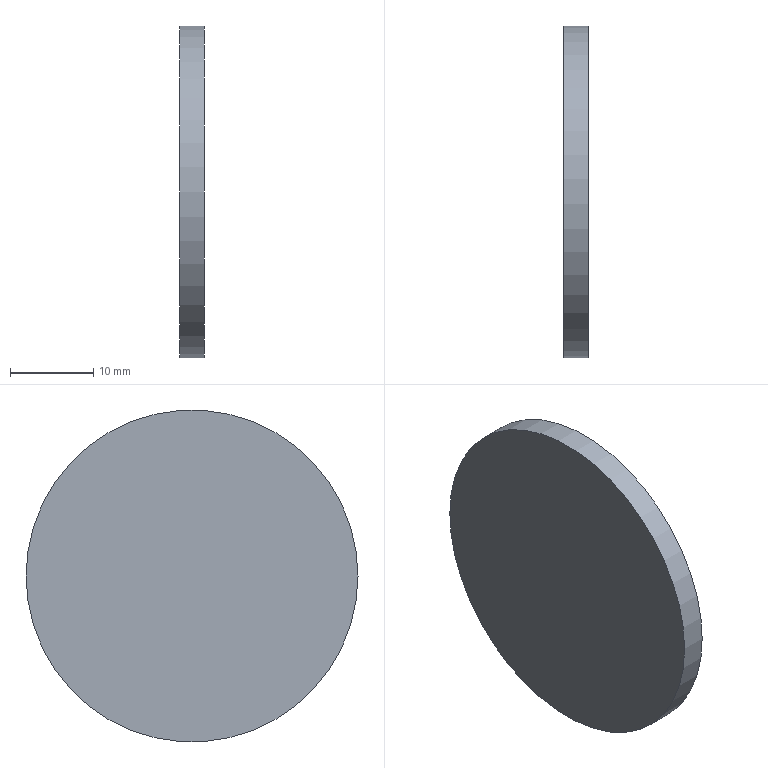Part | NX | features solid 2 | 1 solid | 3 faces | box 3 x 40 x 40 mm | volume 3770 mm3 | plane 2 | cylinder 1 | commonest cylinder face diameters 40 x1
STEP:
#1=CARTESIAN_POINT('',(1112.,-176.,-405.));
#2=VERTEX_POINT('',#1);
#3=CARTESIAN_POINT('',(1112.,-156.,-405.));
#4=DIRECTION('',(1.,0.,0.));
#5=DIRECTION('',(0.,-1.,0.));
#6=AXIS2_PLACEMENT_3D('',#3,#4,#5);
#7=CIRCLE('',#6,20.);
#8=EDGE_CURVE('',#2,#2,#7,.T.);
#9=ORIENTED_EDGE('',*,*,#8,.F.);
#10=EDGE_LOOP('',(#9));
#11=FACE_BOUND('',#10,.T.);
#12=CARTESIAN_POINT('',(1109.,-176.,-405.));
#13=VERTEX_POINT('',#12);
#14=CARTESIAN_POINT('',(1109.,-156.,-405.));
#15=DIRECTION('',(1.,0.,0.));
#16=DIRECTION('',(0.,-1.,0.));
#17=AXIS2_PLACEMENT_3D('',#14,#15,#16);
#18=CIRCLE('',#17,20.);
#19=EDGE_CURVE('',#13,#13,#18,.T.);
#20=ORIENTED_EDGE('',*,*,#19,.T.);
#21=EDGE_LOOP('',(#20));
#22=FACE_BOUND('',#21,.T.);
#23=CARTESIAN_POINT('',(1112.,-156.,-405.));
#24=DIRECTION('',(-1.,0.,0.));
#25=DIRECTION('',(0.,1.,0.));
#26=AXIS2_PLACEMENT_3D('',#23,#24,#25);
#27=CYLINDRICAL_SURFACE('',#26,20.);
#28=ADVANCED_FACE('',(#11,#22),#27,.T.);
#29=ORIENTED_EDGE('',*,*,#8,.T.);
#30=EDGE_LOOP('',(#29));
#31=FACE_BOUND('',#30,.T.);
#32=CARTESIAN_POINT('',(1112.,-156.,-405.));
#33=DIRECTION('',(1.,0.,0.));
#34=DIRECTION('',(0.,-1.,0.));
#35=AXIS2_PLACEMENT_3D('',#32,#33,#34);
#36=PLANE('',#35);
#37=ADVANCED_FACE('',(#31),#36,.T.);
#38=ORIENTED_EDGE('',*,*,#19,.F.);
#39=EDGE_LOOP('',(#38));
#40=FACE_BOUND('',#39,.T.);
#41=CARTESIAN_POINT('',(1109.,-156.,-405.));
#42=DIRECTION('',(1.,0.,0.));
#43=DIRECTION('',(0.,-1.,0.));
#44=AXIS2_PLACEMENT_3D('',#41,#42,#43);
#45=PLANE('',#44);
#46=ADVANCED_FACE('',(#40),#45,.F.);
#47=CLOSED_SHELL('',(#28,#37,#46));
#48=MANIFOLD_SOLID_BREP('',#47);
#49=(LENGTH_UNIT()NAMED_UNIT(*)SI_UNIT(.MILLI.,.METRE.));
#50=UNCERTAINTY_MEASURE_WITH_UNIT(LENGTH_MEASURE(0.00001),#49,'','');
#51=(NAMED_UNIT(*)PLANE_ANGLE_UNIT()SI_UNIT($,.RADIAN.));
#52=(NAMED_UNIT(*)SI_UNIT($,.STERADIAN.)SOLID_ANGLE_UNIT());
#53=(GEOMETRIC_REPRESENTATION_CONTEXT(3)GLOBAL_UNCERTAINTY_ASSIGNED_CONTEXT((#50))GLOBAL_UNIT_ASSIGNED_CONTEXT((#49,#51,#52))REPRESENTATION_CONTEXT('',''));
#54=ADVANCED_BREP_SHAPE_REPRESENTATION('',(#48),#53);